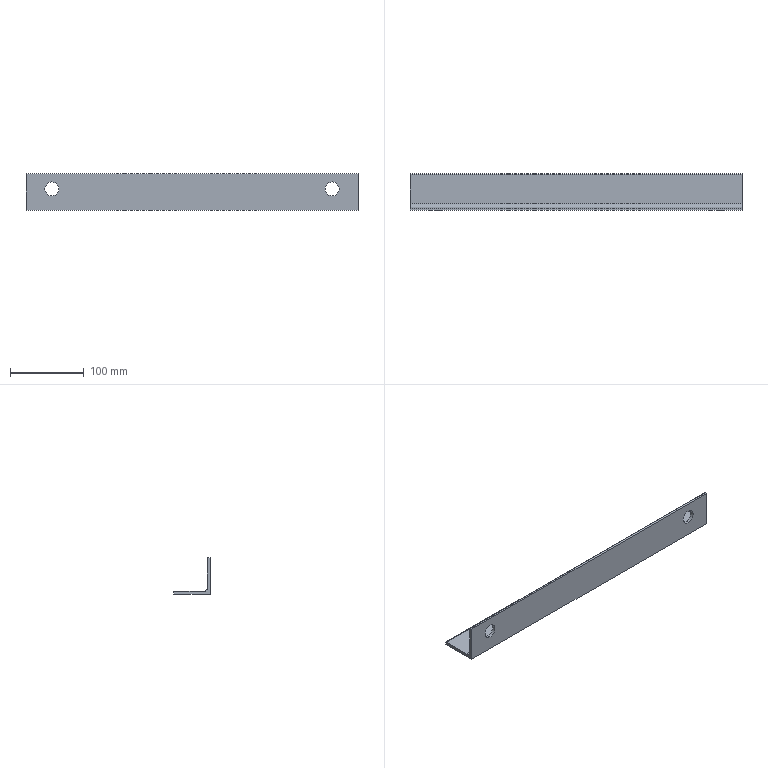Part | STEP file | 计量角钢2_Default<As Machined> | 1 solid | 15 faces | box 450 x 50 x 50 mm | volume 173111 mm3 | plane 8 | cylinder 7 | commonest cylinder face diameters 19 x4 2.66 x2 11 x1
STEP:
#1=CARTESIAN_POINT('',(0.,0.,0.));
#2=DIRECTION('',(0.,0.,1.));
#3=DIRECTION('',(1.,0.,0.));
#4=AXIS2_PLACEMENT_3D('',#1,#2,#3);
#5=CARTESIAN_POINT('',(-190.,0.,38.585));
#6=VERTEX_POINT('',#5);
#7=CARTESIAN_POINT('',(-190.,4.,38.585));
#8=VERTEX_POINT('',#7);
#9=CARTESIAN_POINT('',(-190.,-6.,38.585));
#10=DIRECTION('',(0.,1.,0.));
#11=VECTOR('',#10,1.);
#12=LINE('',#9,#11);
#13=CARTESIAN_POINT('',(-190.,-6.,29.085));
#14=DIRECTION('',(0.,1.,0.));
#15=DIRECTION('',(0.,0.,1.));
#16=AXIS2_PLACEMENT_3D('',#13,#14,#15);
#17=CYLINDRICAL_SURFACE('',#16,9.5);
#18=CARTESIAN_POINT('',(6.283,0.));
#19=DIRECTION('',(0.,1.));
#20=VECTOR('',#19,1.);
#21=LINE('',#18,#20);
#22=(GEOMETRIC_REPRESENTATION_CONTEXT(2)PARAMETRIC_REPRESENTATION_CONTEXT()REPRESENTATION_CONTEXT('',''));
#23=DEFINITIONAL_REPRESENTATION('',(#21),#22);
#24=PCURVE('',#17,#23);
#25=CARTESIAN_POINT('',(-190.,-6.,29.085));
#26=DIRECTION('',(0.,1.,0.));
#27=DIRECTION('',(0.,0.,1.));
#28=AXIS2_PLACEMENT_3D('',#25,#26,#27);
#29=CYLINDRICAL_SURFACE('',#28,9.5);
#30=CARTESIAN_POINT('',(0.,0.));
#31=DIRECTION('',(0.,1.));
#32=VECTOR('',#31,1.);
#33=LINE('',#30,#32);
#34=(GEOMETRIC_REPRESENTATION_CONTEXT(2)PARAMETRIC_REPRESENTATION_CONTEXT()REPRESENTATION_CONTEXT('',''));
#35=DEFINITIONAL_REPRESENTATION('',(#33),#34);
#36=PCURVE('',#29,#35);
#37=SURFACE_CURVE('',#12,(#24,#36),.PCURVE_S1.);
#38=EDGE_CURVE('',#6,#8,#37,.T.);
#39=ORIENTED_EDGE('',*,*,#38,.T.);
#40=CARTESIAN_POINT('',(-190.,4.,19.585));
#41=VERTEX_POINT('',#40);
#42=CARTESIAN_POINT('',(-190.,4.,29.085));
#43=DIRECTION('',(0.,1.,0.));
#44=DIRECTION('',(0.,0.,1.));
#45=AXIS2_PLACEMENT_3D('',#42,#43,#44);
#46=CIRCLE('',#45,9.5);
#47=CARTESIAN_POINT('',(0.,10.));
#48=DIRECTION('',(1.,0.));
#49=VECTOR('',#48,1.);
#50=LINE('',#47,#49);
#51=(GEOMETRIC_REPRESENTATION_CONTEXT(2)PARAMETRIC_REPRESENTATION_CONTEXT()REPRESENTATION_CONTEXT('',''));
#52=DEFINITIONAL_REPRESENTATION('',(#50),#51);
#53=PCURVE('',#17,#52);
#54=CARTESIAN_POINT('',(225.,4.,48.67));
#55=DIRECTION('',(0.,-1.,0.));
#56=DIRECTION('',(1.,0.,0.));
#57=AXIS2_PLACEMENT_3D('',#54,#55,#56);
#58=PLANE('',#57);
#59=CARTESIAN_POINT('',(-415.,-10.085));
#60=CARTESIAN_POINT('',(-398.546,-10.085));
#61=CARTESIAN_POINT('',(-406.773,-24.335));
#62=CARTESIAN_POINT('',(-415.,-38.585));
#63=CARTESIAN_POINT('',(-423.227,-24.335));
#64=CARTESIAN_POINT('',(-431.454,-10.085));
#65=CARTESIAN_POINT('',(-415.,-10.085));
#66=(BOUNDED_CURVE()B_SPLINE_CURVE(2,(#59,#60,#61,#62,#63,#64,#65),.UNSPECIFIED.,.T.,.F.)B_SPLINE_CURVE_WITH_KNOTS((1,2,2,2,2,1),(-2.094,0.,2.094,4.189,6.283,8.378),.UNSPECIFIED.)CURVE()GEOMETRIC_REPRESENTATION_ITEM()RATIONAL_B_SPLINE_CURVE((1.,0.5,1.,0.5,1.,0.5,1.))REPRESENTATION_ITEM(''));
#67=(GEOMETRIC_REPRESENTATION_CONTEXT(2)PARAMETRIC_REPRESENTATION_CONTEXT()REPRESENTATION_CONTEXT('',''));
#68=DEFINITIONAL_REPRESENTATION('',(#66),#67);
#69=PCURVE('',#58,#68);
#70=SURFACE_CURVE('',#46,(#53,#69),.PCURVE_S1.);
#71=EDGE_CURVE('',#41,#8,#70,.T.);
#72=ORIENTED_EDGE('',*,*,#71,.F.);
#73=CARTESIAN_POINT('',(-190.,0.,19.585));
#74=VERTEX_POINT('',#73);
#75=CARTESIAN_POINT('',(-190.,-6.,19.585));
#76=DIRECTION('',(0.,1.,0.));
#77=VECTOR('',#76,1.);
#78=LINE('',#75,#77);
#79=CARTESIAN_POINT('',(3.142,0.));
#80=DIRECTION('',(0.,1.));
#81=VECTOR('',#80,1.);
#82=LINE('',#79,#81);
#83=(GEOMETRIC_REPRESENTATION_CONTEXT(2)PARAMETRIC_REPRESENTATION_CONTEXT()REPRESENTATION_CONTEXT('',''));
#84=DEFINITIONAL_REPRESENTATION('',(#82),#83);
#85=PCURVE('',#17,#84);
#86=CARTESIAN_POINT('',(3.142,0.));
#87=DIRECTION('',(0.,1.));
#88=VECTOR('',#87,1.);
#89=LINE('',#86,#88);
#90=(GEOMETRIC_REPRESENTATION_CONTEXT(2)PARAMETRIC_REPRESENTATION_CONTEXT()REPRESENTATION_CONTEXT('',''));
#91=DEFINITIONAL_REPRESENTATION('',(#89),#90);
#92=PCURVE('',#29,#91);
#93=SURFACE_CURVE('',#78,(#85,#92),.PCURVE_S1.);
#94=EDGE_CURVE('',#74,#41,#93,.T.);
#95=ORIENTED_EDGE('',*,*,#94,.F.);
#96=CARTESIAN_POINT('',(-190.,0.,29.085));
#97=DIRECTION('',(0.,1.,0.));
#98=DIRECTION('',(-1.,0.,0.));
#99=AXIS2_PLACEMENT_3D('',#96,#97,#98);
#100=CIRCLE('',#99,9.5);
#101=CARTESIAN_POINT('',(-1.571,6.));
#102=DIRECTION('',(1.,0.));
#103=VECTOR('',#102,1.);
#104=LINE('',#101,#103);
#105=(GEOMETRIC_REPRESENTATION_CONTEXT(2)PARAMETRIC_REPRESENTATION_CONTEXT()REPRESENTATION_CONTEXT('',''));
#106=DEFINITIONAL_REPRESENTATION('',(#104),#105);
#107=PCURVE('',#17,#106);
#108=CARTESIAN_POINT('',(225.,0.,50.));
#109=DIRECTION('',(0.,1.,0.));
#110=DIRECTION('',(-1.,0.,0.));
#111=AXIS2_PLACEMENT_3D('',#108,#109,#110);
#112=PLANE('',#111);
#113=CARTESIAN_POINT('',(415.,-20.915));
#114=DIRECTION('',(1.,0.));
#115=AXIS2_PLACEMENT_2D('',#113,#114);
#116=CIRCLE('',#115,9.5);
#117=(GEOMETRIC_REPRESENTATION_CONTEXT(2)PARAMETRIC_REPRESENTATION_CONTEXT()REPRESENTATION_CONTEXT('',''));
#118=DEFINITIONAL_REPRESENTATION('',(#116),#117);
#119=PCURVE('',#112,#118);
#120=SURFACE_CURVE('',#100,(#107,#119),.PCURVE_S1.);
#121=EDGE_CURVE('',#74,#6,#120,.T.);
#122=ORIENTED_EDGE('',*,*,#121,.T.);
#123=EDGE_LOOP('',(#39,#72,#95,#122));
#124=FACE_BOUND('',#123,.F.);
#125=ADVANCED_FACE('',(#124),#17,.F.);
#126=CARTESIAN_POINT('',(190.,0.,38.585));
#127=VERTEX_POINT('',#126);
#128=CARTESIAN_POINT('',(190.,4.,38.585));
#129=VERTEX_POINT('',#128);
#130=CARTESIAN_POINT('',(190.,-6.,38.585));
#131=DIRECTION('',(0.,1.,0.));
#132=VECTOR('',#131,1.);
#133=LINE('',#130,#132);
#134=CARTESIAN_POINT('',(190.,-6.,29.085));
#135=DIRECTION('',(0.,1.,0.));
#136=DIRECTION('',(0.,0.,1.));
#137=AXIS2_PLACEMENT_3D('',#134,#135,#136);
#138=CYLINDRICAL_SURFACE('',#137,9.5);
#139=CARTESIAN_POINT('',(6.283,0.));
#140=DIRECTION('',(0.,1.));
#141=VECTOR('',#140,1.);
#142=LINE('',#139,#141);
#143=(GEOMETRIC_REPRESENTATION_CONTEXT(2)PARAMETRIC_REPRESENTATION_CONTEXT()REPRESENTATION_CONTEXT('',''));
#144=DEFINITIONAL_REPRESENTATION('',(#142),#143);
#145=PCURVE('',#138,#144);
#146=CARTESIAN_POINT('',(190.,-6.,29.085));
#147=DIRECTION('',(0.,1.,0.));
#148=DIRECTION('',(0.,0.,1.));
#149=AXIS2_PLACEMENT_3D('',#146,#147,#148);
#150=CYLINDRICAL_SURFACE('',#149,9.5);
#151=CARTESIAN_POINT('',(0.,0.));
#152=DIRECTION('',(0.,1.));
#153=VECTOR('',#152,1.);
#154=LINE('',#151,#153);
#155=(GEOMETRIC_REPRESENTATION_CONTEXT(2)PARAMETRIC_REPRESENTATION_CONTEXT()REPRESENTATION_CONTEXT('',''));
#156=DEFINITIONAL_REPRESENTATION('',(#154),#155);
#157=PCURVE('',#150,#156);
#158=SURFACE_CURVE('',#133,(#145,#157),.PCURVE_S1.);
#159=EDGE_CURVE('',#127,#129,#158,.T.);
#160=ORIENTED_EDGE('',*,*,#159,.T.);
#161=CARTESIAN_POINT('',(190.,4.,19.585));
#162=VERTEX_POINT('',#161);
#163=CARTESIAN_POINT('',(190.,4.,29.085));
#164=DIRECTION('',(0.,1.,0.));
#165=DIRECTION('',(0.,0.,-1.));
#166=AXIS2_PLACEMENT_3D('',#163,#164,#165);
#167=CIRCLE('',#166,9.5);
#168=CARTESIAN_POINT('',(3.142,10.));
#169=DIRECTION('',(1.,0.));
#170=VECTOR('',#169,1.);
#171=LINE('',#168,#170);
#172=(GEOMETRIC_REPRESENTATION_CONTEXT(2)PARAMETRIC_REPRESENTATION_CONTEXT()REPRESENTATION_CONTEXT('',''));
#173=DEFINITIONAL_REPRESENTATION('',(#171),#172);
#174=PCURVE('',#138,#173);
#175=CARTESIAN_POINT('',(-35.,-29.085));
#176=CARTESIAN_POINT('',(-51.454,-29.085));
#177=CARTESIAN_POINT('',(-43.227,-14.835));
#178=CARTESIAN_POINT('',(-35.,-0.585));
#179=CARTESIAN_POINT('',(-26.773,-14.835));
#180=CARTESIAN_POINT('',(-18.546,-29.085));
#181=CARTESIAN_POINT('',(-35.,-29.085));
#182=(BOUNDED_CURVE()B_SPLINE_CURVE(2,(#175,#176,#177,#178,#179,#180,#181),.UNSPECIFIED.,.T.,.F.)B_SPLINE_CURVE_WITH_KNOTS((1,2,2,2,2,1),(-2.094,0.,2.094,4.189,6.283,8.378),.UNSPECIFIED.)CURVE()GEOMETRIC_REPRESENTATION_ITEM()RATIONAL_B_SPLINE_CURVE((1.,0.5,1.,0.5,1.,0.5,1.))REPRESENTATION_ITEM(''));
#183=(GEOMETRIC_REPRESENTATION_CONTEXT(2)PARAMETRIC_REPRESENTATION_CONTEXT()REPRESENTATION_CONTEXT('',''));
#184=DEFINITIONAL_REPRESENTATION('',(#182),#183);
#185=PCURVE('',#58,#184);
#186=SURFACE_CURVE('',#167,(#174,#185),.PCURVE_S1.);
#187=EDGE_CURVE('',#162,#129,#186,.T.);
#188=ORIENTED_EDGE('',*,*,#187,.F.);
#189=CARTESIAN_POINT('',(190.,0.,19.585));
#190=VERTEX_POINT('',#189);
#191=CARTESIAN_POINT('',(190.,-6.,19.585));
#192=DIRECTION('',(0.,1.,0.));
#193=VECTOR('',#192,1.);
#194=LINE('',#191,#193);
#195=CARTESIAN_POINT('',(3.142,0.));
#196=DIRECTION('',(0.,1.));
#197=VECTOR('',#196,1.);
#198=LINE('',#195,#197);
#199=(GEOMETRIC_REPRESENTATION_CONTEXT(2)PARAMETRIC_REPRESENTATION_CONTEXT()REPRESENTATION_CONTEXT('',''));
#200=DEFINITIONAL_REPRESENTATION('',(#198),#199);
#201=PCURVE('',#138,#200);
#202=CARTESIAN_POINT('',(3.142,0.));
#203=DIRECTION('',(0.,1.));
#204=VECTOR('',#203,1.);
#205=LINE('',#202,#204);
#206=(GEOMETRIC_REPRESENTATION_CONTEXT(2)PARAMETRIC_REPRESENTATION_CONTEXT()REPRESENTATION_CONTEXT('',''));
#207=DEFINITIONAL_REPRESENTATION('',(#205),#206);
#208=PCURVE('',#150,#207);
#209=SURFACE_CURVE('',#194,(#201,#208),.PCURVE_S1.);
#210=EDGE_CURVE('',#190,#162,#209,.T.);
#211=ORIENTED_EDGE('',*,*,#210,.F.);
#212=CARTESIAN_POINT('',(190.,0.,29.085));
#213=DIRECTION('',(0.,1.,0.));
#214=DIRECTION('',(-1.,0.,0.));
#215=AXIS2_PLACEMENT_3D('',#212,#213,#214);
#216=CIRCLE('',#215,9.5);
#217=CARTESIAN_POINT('',(-1.571,6.));
#218=DIRECTION('',(1.,0.));
#219=VECTOR('',#218,1.);
#220=LINE('',#217,#219);
#221=(GEOMETRIC_REPRESENTATION_CONTEXT(2)PARAMETRIC_REPRESENTATION_CONTEXT()REPRESENTATION_CONTEXT('',''));
#222=DEFINITIONAL_REPRESENTATION('',(#220),#221);
#223=PCURVE('',#138,#222);
#224=CARTESIAN_POINT('',(35.,-20.915));
#225=DIRECTION('',(1.,0.));
#226=AXIS2_PLACEMENT_2D('',#224,#225);
#227=CIRCLE('',#226,9.5);
#228=(GEOMETRIC_REPRESENTATION_CONTEXT(2)PARAMETRIC_REPRESENTATION_CONTEXT()REPRESENTATION_CONTEXT('',''));
#229=DEFINITIONAL_REPRESENTATION('',(#227),#228);
#230=PCURVE('',#112,#229);
#231=SURFACE_CURVE('',#216,(#223,#230),.PCURVE_S1.);
#232=EDGE_CURVE('',#190,#127,#231,.T.);
#233=ORIENTED_EDGE('',*,*,#232,.T.);
#234=EDGE_LOOP('',(#160,#188,#211,#233));
#235=FACE_BOUND('',#234,.F.);
#236=ADVANCED_FACE('',(#235),#138,.F.);
#237=CARTESIAN_POINT('',(-225.,50.,2.67));
#238=VERTEX_POINT('',#237);
#239=CARTESIAN_POINT('',(-225.,48.67,4.));
#240=VERTEX_POINT('',#239);
#241=CARTESIAN_POINT('',(-225.,48.67,2.67));
#242=DIRECTION('',(1.,0.,0.));
#243=DIRECTION('',(0.,1.,0.));
#244=AXIS2_PLACEMENT_3D('',#241,#242,#243);
#245=CIRCLE('',#244,1.33);
#246=CARTESIAN_POINT('',(225.,48.67,2.67));
#247=DIRECTION('',(-1.,0.,0.));
#248=DIRECTION('',(0.,-1.,0.));
#249=AXIS2_PLACEMENT_3D('',#246,#247,#248);
#250=CYLINDRICAL_SURFACE('',#249,1.33);
#251=CARTESIAN_POINT('',(3.142,450.));
#252=DIRECTION('',(-1.,0.));
#253=VECTOR('',#252,1.);
#254=LINE('',#251,#253);
#255=(GEOMETRIC_REPRESENTATION_CONTEXT(2)PARAMETRIC_REPRESENTATION_CONTEXT()REPRESENTATION_CONTEXT('',''));
#256=DEFINITIONAL_REPRESENTATION('',(#254),#255);
#257=PCURVE('',#250,#256);
#258=CARTESIAN_POINT('',(-225.,48.67,2.67));
#259=DIRECTION('',(1.,0.,0.));
#260=DIRECTION('',(0.,1.,0.));
#261=AXIS2_PLACEMENT_3D('',#258,#259,#260);
#262=PLANE('',#261);
#263=CARTESIAN_POINT('',(0.,0.));
#264=DIRECTION('',(1.,0.));
#265=AXIS2_PLACEMENT_2D('',#263,#264);
#266=CIRCLE('',#265,1.33);
#267=(GEOMETRIC_REPRESENTATION_CONTEXT(2)PARAMETRIC_REPRESENTATION_CONTEXT()REPRESENTATION_CONTEXT('',''));
#268=DEFINITIONAL_REPRESENTATION('',(#266),#267);
#269=PCURVE('',#262,#268);
#270=SURFACE_CURVE('',#245,(#257,#269),.PCURVE_S1.);
#271=EDGE_CURVE('',#238,#240,#270,.T.);
#272=ORIENTED_EDGE('',*,*,#271,.T.);
#273=CARTESIAN_POINT('',(225.,48.67,4.));
#274=VERTEX_POINT('',#273);
#275=CARTESIAN_POINT('',(225.,48.67,4.));
#276=DIRECTION('',(-1.,0.,0.));
#277=VECTOR('',#276,1.);
#278=LINE('',#275,#277);
#279=CARTESIAN_POINT('',(1.571,0.));
#280=DIRECTION('',(0.,1.));
#281=VECTOR('',#280,1.);
#282=LINE('',#279,#281);
#283=(GEOMETRIC_REPRESENTATION_CONTEXT(2)PARAMETRIC_REPRESENTATION_CONTEXT()REPRESENTATION_CONTEXT('',''));
#284=DEFINITIONAL_REPRESENTATION('',(#282),#283);
#285=PCURVE('',#250,#284);
#286=CARTESIAN_POINT('',(225.,9.5,4.));
#287=DIRECTION('',(0.,0.,-1.));
#288=DIRECTION('',(-1.,0.,0.));
#289=AXIS2_PLACEMENT_3D('',#286,#287,#288);
#290=PLANE('',#289);
#291=CARTESIAN_POINT('',(0.,39.17));
#292=DIRECTION('',(1.,0.));
#293=VECTOR('',#292,1.);
#294=LINE('',#291,#293);
#295=(GEOMETRIC_REPRESENTATION_CONTEXT(2)PARAMETRIC_REPRESENTATION_CONTEXT()REPRESENTATION_CONTEXT('',''));
#296=DEFINITIONAL_REPRESENTATION('',(#294),#295);
#297=PCURVE('',#290,#296);
#298=SURFACE_CURVE('',#278,(#285,#297),.PCURVE_S1.);
#299=EDGE_CURVE('',#274,#240,#298,.T.);
#300=ORIENTED_EDGE('',*,*,#299,.F.);
#301=CARTESIAN_POINT('',(225.,50.,2.67));
#302=VERTEX_POINT('',#301);
#303=CARTESIAN_POINT('',(225.,48.67,2.67));
#304=DIRECTION('',(1.,0.,0.));
#305=DIRECTION('',(0.,1.,0.));
#306=AXIS2_PLACEMENT_3D('',#303,#304,#305);
#307=CIRCLE('',#306,1.33);
#308=CARTESIAN_POINT('',(3.142,0.));
#309=DIRECTION('',(-1.,0.));
#310=VECTOR('',#309,1.);
#311=LINE('',#308,#310);
#312=(GEOMETRIC_REPRESENTATION_CONTEXT(2)PARAMETRIC_REPRESENTATION_CONTEXT()REPRESENTATION_CONTEXT('',''));
#313=DEFINITIONAL_REPRESENTATION('',(#311),#312);
#314=PCURVE('',#250,#313);
#315=CARTESIAN_POINT('',(225.,48.67,2.67));
#316=DIRECTION('',(1.,0.,0.));
#317=DIRECTION('',(0.,1.,0.));
#318=AXIS2_PLACEMENT_3D('',#315,#316,#317);
#319=PLANE('',#318);
#320=CARTESIAN_POINT('',(0.,0.));
#321=DIRECTION('',(1.,0.));
#322=AXIS2_PLACEMENT_2D('',#320,#321);
#323=CIRCLE('',#322,1.33);
#324=(GEOMETRIC_REPRESENTATION_CONTEXT(2)PARAMETRIC_REPRESENTATION_CONTEXT()REPRESENTATION_CONTEXT('',''));
#325=DEFINITIONAL_REPRESENTATION('',(#323),#324);
#326=PCURVE('',#319,#325);
#327=SURFACE_CURVE('',#307,(#314,#326),.PCURVE_S1.);
#328=EDGE_CURVE('',#302,#274,#327,.T.);
#329=ORIENTED_EDGE('',*,*,#328,.F.);
#330=CARTESIAN_POINT('',(225.,50.,2.67));
#331=DIRECTION('',(-1.,0.,0.));
#332=VECTOR('',#331,1.);
#333=LINE('',#330,#332);
#334=CARTESIAN_POINT('',(3.142,0.));
#335=DIRECTION('',(0.,1.));
#336=VECTOR('',#335,1.);
#337=LINE('',#334,#336);
#338=(GEOMETRIC_REPRESENTATION_CONTEXT(2)PARAMETRIC_REPRESENTATION_CONTEXT()REPRESENTATION_CONTEXT('',''));
#339=DEFINITIONAL_REPRESENTATION('',(#337),#338);
#340=PCURVE('',#250,#339);
#341=CARTESIAN_POINT('',(225.,50.,2.67));
#342=DIRECTION('',(0.,-1.,0.));
#343=DIRECTION('',(1.,0.,0.));
#344=AXIS2_PLACEMENT_3D('',#341,#342,#343);
#345=PLANE('',#344);
#346=CARTESIAN_POINT('',(0.,0.));
#347=DIRECTION('',(-1.,0.));
#348=VECTOR('',#347,1.);
#349=LINE('',#346,#348);
#350=(GEOMETRIC_REPRESENTATION_CONTEXT(2)PARAMETRIC_REPRESENTATION_CONTEXT()REPRESENTATION_CONTEXT('',''));
#351=DEFINITIONAL_REPRESENTATION('',(#349),#350);
#352=PCURVE('',#345,#351);
#353=SURFACE_CURVE('',#333,(#340,#352),.PCURVE_S1.);
#354=EDGE_CURVE('',#302,#238,#353,.T.);
#355=ORIENTED_EDGE('',*,*,#354,.T.);
#356=EDGE_LOOP('',(#272,#300,#329,#355));
#357=FACE_BOUND('',#356,.T.);
#358=ADVANCED_FACE('',(#357),#250,.T.);
#359=CARTESIAN_POINT('',(-225.,9.5,4.));
#360=VERTEX_POINT('',#359);
#361=CARTESIAN_POINT('',(-225.,9.5,4.));
#362=DIRECTION('',(0.,-1.,0.));
#363=VECTOR('',#362,1.);
#364=LINE('',#361,#363);
#365=CARTESIAN_POINT('',(450.,0.));
#366=DIRECTION('',(0.,-1.));
#367=VECTOR('',#366,1.);
#368=LINE('',#365,#367);
#369=(GEOMETRIC_REPRESENTATION_CONTEXT(2)PARAMETRIC_REPRESENTATION_CONTEXT()REPRESENTATION_CONTEXT('',''));
#370=DEFINITIONAL_REPRESENTATION('',(#368),#369);
#371=PCURVE('',#290,#370);
#372=CARTESIAN_POINT('',(-39.17,1.33));
#373=DIRECTION('',(-1.,0.));
#374=VECTOR('',#373,1.);
#375=LINE('',#372,#374);
#376=(GEOMETRIC_REPRESENTATION_CONTEXT(2)PARAMETRIC_REPRESENTATION_CONTEXT()REPRESENTATION_CONTEXT('',''));
#377=DEFINITIONAL_REPRESENTATION('',(#375),#376);
#378=PCURVE('',#262,#377);
#379=SURFACE_CURVE('',#364,(#371,#378),.PCURVE_S1.);
#380=EDGE_CURVE('',#240,#360,#379,.T.);
#381=ORIENTED_EDGE('',*,*,#380,.T.);
#382=CARTESIAN_POINT('',(225.,9.5,4.));
#383=VERTEX_POINT('',#382);
#384=CARTESIAN_POINT('',(225.,9.5,4.));
#385=DIRECTION('',(-1.,0.,0.));
#386=VECTOR('',#385,1.);
#387=LINE('',#384,#386);
#388=CARTESIAN_POINT('',(0.,0.));
#389=DIRECTION('',(1.,0.));
#390=VECTOR('',#389,1.);
#391=LINE('',#388,#390);
#392=(GEOMETRIC_REPRESENTATION_CONTEXT(2)PARAMETRIC_REPRESENTATION_CONTEXT()REPRESENTATION_CONTEXT('',''));
#393=DEFINITIONAL_REPRESENTATION('',(#391),#392);
#394=PCURVE('',#290,#393);
#395=CARTESIAN_POINT('',(225.,9.5,9.5));
#396=DIRECTION('',(-1.,0.,0.));
#397=DIRECTION('',(0.,-1.,0.));
#398=AXIS2_PLACEMENT_3D('',#395,#396,#397);
#399=CYLINDRICAL_SURFACE('',#398,5.5);
#400=CARTESIAN_POINT('',(4.712,0.));
#401=DIRECTION('',(0.,1.));
#402=VECTOR('',#401,1.);
#403=LINE('',#400,#402);
#404=(GEOMETRIC_REPRESENTATION_CONTEXT(2)PARAMETRIC_REPRESENTATION_CONTEXT()REPRESENTATION_CONTEXT('',''));
#405=DEFINITIONAL_REPRESENTATION('',(#403),#404);
#406=PCURVE('',#399,#405);
#407=SURFACE_CURVE('',#387,(#394,#406),.PCURVE_S1.);
#408=EDGE_CURVE('',#383,#360,#407,.T.);
#409=ORIENTED_EDGE('',*,*,#408,.F.);
#410=CARTESIAN_POINT('',(225.,9.5,4.));
#411=DIRECTION('',(0.,-1.,0.));
#412=VECTOR('',#411,1.);
#413=LINE('',#410,#412);
#414=CARTESIAN_POINT('',(0.,0.));
#415=DIRECTION('',(0.,-1.));
#416=VECTOR('',#415,1.);
#417=LINE('',#414,#416);
#418=(GEOMETRIC_REPRESENTATION_CONTEXT(2)PARAMETRIC_REPRESENTATION_CONTEXT()REPRESENTATION_CONTEXT('',''));
#419=DEFINITIONAL_REPRESENTATION('',(#417),#418);
#420=PCURVE('',#290,#419);
#421=CARTESIAN_POINT('',(-39.17,1.33));
#422=DIRECTION('',(-1.,0.));
#423=VECTOR('',#422,1.);
#424=LINE('',#421,#423);
#425=(GEOMETRIC_REPRESENTATION_CONTEXT(2)PARAMETRIC_REPRESENTATION_CONTEXT()REPRESENTATION_CONTEXT('',''));
#426=DEFINITIONAL_REPRESENTATION('',(#424),#425);
#427=PCURVE('',#319,#426);
#428=SURFACE_CURVE('',#413,(#420,#427),.PCURVE_S1.);
#429=EDGE_CURVE('',#274,#383,#428,.T.);
#430=ORIENTED_EDGE('',*,*,#429,.F.);
#431=ORIENTED_EDGE('',*,*,#299,.T.);
#432=EDGE_LOOP('',(#381,#409,#430,#431));
#433=FACE_BOUND('',#432,.T.);
#434=ADVANCED_FACE('',(#433),#290,.F.);
#435=ORIENTED_EDGE('',*,*,#408,.F.);
#436=CARTESIAN_POINT('',(225.,4.,9.5));
#437=VERTEX_POINT('',#436);
#438=CARTESIAN_POINT('',(225.,9.5,9.5));
#439=DIRECTION('',(-1.,0.,0.));
#440=DIRECTION('',(0.,1.,0.));
#441=AXIS2_PLACEMENT_3D('',#438,#439,#440);
#442=CIRCLE('',#441,5.5);
#443=CARTESIAN_POINT('',(3.142,0.));
#444=DIRECTION('',(1.,0.));
#445=VECTOR('',#444,1.);
#446=LINE('',#443,#445);
#447=(GEOMETRIC_REPRESENTATION_CONTEXT(2)PARAMETRIC_REPRESENTATION_CONTEXT()REPRESENTATION_CONTEXT('',''));
#448=DEFINITIONAL_REPRESENTATION('',(#446),#447);
#449=PCURVE('',#399,#448);
#450=CARTESIAN_POINT('',(-33.67,6.83));
#451=CARTESIAN_POINT('',(-33.67,-2.696));
#452=CARTESIAN_POINT('',(-41.92,2.067));
#453=CARTESIAN_POINT('',(-50.17,6.83));
#454=CARTESIAN_POINT('',(-41.92,11.593));
#455=CARTESIAN_POINT('',(-33.67,16.356));
#456=CARTESIAN_POINT('',(-33.67,6.83));
#457=(BOUNDED_CURVE()B_SPLINE_CURVE(2,(#450,#451,#452,#453,#454,#455,#456),.UNSPECIFIED.,.T.,.F.)B_SPLINE_CURVE_WITH_KNOTS((1,2,2,2,2,1),(-2.094,0.,2.094,4.189,6.283,8.378),.UNSPECIFIED.)CURVE()GEOMETRIC_REPRESENTATION_ITEM()RATIONAL_B_SPLINE_CURVE((1.,0.5,1.,0.5,1.,0.5,1.))REPRESENTATION_ITEM(''));
#458=(GEOMETRIC_REPRESENTATION_CONTEXT(2)PARAMETRIC_REPRESENTATION_CONTEXT()REPRESENTATION_CONTEXT('',''));
#459=DEFINITIONAL_REPRESENTATION('',(#457),#458);
#460=PCURVE('',#319,#459);
#461=SURFACE_CURVE('',#442,(#449,#460),.PCURVE_S1.);
#462=EDGE_CURVE('',#383,#437,#461,.T.);
#463=ORIENTED_EDGE('',*,*,#462,.T.);
#464=CARTESIAN_POINT('',(-225.,4.,9.5));
#465=VERTEX_POINT('',#464);
#466=CARTESIAN_POINT('',(225.,4.,9.5));
#467=DIRECTION('',(-1.,0.,0.));
#468=VECTOR('',#467,1.);
#469=LINE('',#466,#468);
#470=CARTESIAN_POINT('',(6.283,0.));
#471=DIRECTION('',(0.,1.));
#472=VECTOR('',#471,1.);
#473=LINE('',#470,#472);
#474=(GEOMETRIC_REPRESENTATION_CONTEXT(2)PARAMETRIC_REPRESENTATION_CONTEXT()REPRESENTATION_CONTEXT('',''));
#475=DEFINITIONAL_REPRESENTATION('',(#473),#474);
#476=PCURVE('',#399,#475);
#477=CARTESIAN_POINT('',(0.,-39.17));
#478=DIRECTION('',(-1.,0.));
#479=VECTOR('',#478,1.);
#480=LINE('',#477,#479);
#481=(GEOMETRIC_REPRESENTATION_CONTEXT(2)PARAMETRIC_REPRESENTATION_CONTEXT()REPRESENTATION_CONTEXT('',''));
#482=DEFINITIONAL_REPRESENTATION('',(#480),#481);
#483=PCURVE('',#58,#482);
#484=SURFACE_CURVE('',#469,(#476,#483),.PCURVE_S1.);
#485=EDGE_CURVE('',#437,#465,#484,.T.);
#486=ORIENTED_EDGE('',*,*,#485,.T.);
#487=CARTESIAN_POINT('',(-225.,9.5,9.5));
#488=DIRECTION('',(-1.,0.,0.));
#489=DIRECTION('',(0.,1.,0.));
#490=AXIS2_PLACEMENT_3D('',#487,#488,#489);
#491=CIRCLE('',#490,5.5);
#492=CARTESIAN_POINT('',(3.142,450.));
#493=DIRECTION('',(1.,0.));
#494=VECTOR('',#493,1.);
#495=LINE('',#492,#494);
#496=(GEOMETRIC_REPRESENTATION_CONTEXT(2)PARAMETRIC_REPRESENTATION_CONTEXT()REPRESENTATION_CONTEXT('',''));
#497=DEFINITIONAL_REPRESENTATION('',(#495),#496);
#498=PCURVE('',#399,#497);
#499=CARTESIAN_POINT('',(-33.67,6.83));
#500=CARTESIAN_POINT('',(-33.67,-2.696));
#501=CARTESIAN_POINT('',(-41.92,2.067));
#502=CARTESIAN_POINT('',(-50.17,6.83));
#503=CARTESIAN_POINT('',(-41.92,11.593));
#504=CARTESIAN_POINT('',(-33.67,16.356));
#505=CARTESIAN_POINT('',(-33.67,6.83));
#506=(BOUNDED_CURVE()B_SPLINE_CURVE(2,(#499,#500,#501,#502,#503,#504,#505),.UNSPECIFIED.,.T.,.F.)B_SPLINE_CURVE_WITH_KNOTS((1,2,2,2,2,1),(-2.094,0.,2.094,4.189,6.283,8.378),.UNSPECIFIED.)CURVE()GEOMETRIC_REPRESENTATION_ITEM()RATIONAL_B_SPLINE_CURVE((1.,0.5,1.,0.5,1.,0.5,1.))REPRESENTATION_ITEM(''));
#507=(GEOMETRIC_REPRESENTATION_CONTEXT(2)PARAMETRIC_REPRESENTATION_CONTEXT()REPRESENTATION_CONTEXT('',''));
#508=DEFINITIONAL_REPRESENTATION('',(#506),#507);
#509=PCURVE('',#262,#508);
#510=SURFACE_CURVE('',#491,(#498,#509),.PCURVE_S1.);
#511=EDGE_CURVE('',#360,#465,#510,.T.);
#512=ORIENTED_EDGE('',*,*,#511,.F.);
#513=EDGE_LOOP('',(#435,#463,#486,#512));
#514=FACE_BOUND('',#513,.F.);
#515=ADVANCED_FACE('',(#514),#399,.F.);
#516=CARTESIAN_POINT('',(-190.,4.,29.085));
#517=DIRECTION('',(0.,1.,0.));
#518=DIRECTION('',(0.,0.,1.));
#519=AXIS2_PLACEMENT_3D('',#516,#517,#518);
#520=CIRCLE('',#519,9.5);
#521=CARTESIAN_POINT('',(-415.,-10.085));
#522=CARTESIAN_POINT('',(-398.546,-10.085));
#523=CARTESIAN_POINT('',(-406.773,-24.335));
#524=CARTESIAN_POINT('',(-415.,-38.585));
#525=CARTESIAN_POINT('',(-423.227,-24.335));
#526=CARTESIAN_POINT('',(-431.454,-10.085));
#527=CARTESIAN_POINT('',(-415.,-10.085));
#528=(BOUNDED_CURVE()B_SPLINE_CURVE(2,(#521,#522,#523,#524,#525,#526,#527),.UNSPECIFIED.,.T.,.F.)B_SPLINE_CURVE_WITH_KNOTS((1,2,2,2,2,1),(-2.094,0.,2.094,4.189,6.283,8.378),.UNSPECIFIED.)CURVE()GEOMETRIC_REPRESENTATION_ITEM()RATIONAL_B_SPLINE_CURVE((1.,0.5,1.,0.5,1.,0.5,1.))REPRESENTATION_ITEM(''));
#529=(GEOMETRIC_REPRESENTATION_CONTEXT(2)PARAMETRIC_REPRESENTATION_CONTEXT()REPRESENTATION_CONTEXT('',''));
#530=DEFINITIONAL_REPRESENTATION('',(#528),#529);
#531=PCURVE('',#58,#530);
#532=CARTESIAN_POINT('',(0.,10.));
#533=DIRECTION('',(1.,0.));
#534=VECTOR('',#533,1.);
#535=LINE('',#532,#534);
#536=(GEOMETRIC_REPRESENTATION_CONTEXT(2)PARAMETRIC_REPRESENTATION_CONTEXT()REPRESENTATION_CONTEXT('',''));
#537=DEFINITIONAL_REPRESENTATION('',(#535),#536);
#538=PCURVE('',#29,#537);
#539=SURFACE_CURVE('',#520,(#531,#538),.PCURVE_S1.);
#540=EDGE_CURVE('',#8,#41,#539,.T.);
#541=ORIENTED_EDGE('',*,*,#540,.F.);
#542=ORIENTED_EDGE('',*,*,#71,.F.);
#543=EDGE_LOOP('',(#541,#542));
#544=FACE_BOUND('',#543,.T.);
#545=CARTESIAN_POINT('',(190.,4.,29.085));
#546=DIRECTION('',(0.,1.,0.));
#547=DIRECTION('',(0.,0.,-1.));
#548=AXIS2_PLACEMENT_3D('',#545,#546,#547);
#549=CIRCLE('',#548,9.5);
#550=CARTESIAN_POINT('',(-35.,-29.085));
#551=CARTESIAN_POINT('',(-51.454,-29.085));
#552=CARTESIAN_POINT('',(-43.227,-14.835));
#553=CARTESIAN_POINT('',(-35.,-0.585));
#554=CARTESIAN_POINT('',(-26.773,-14.835));
#555=CARTESIAN_POINT('',(-18.546,-29.085));
#556=CARTESIAN_POINT('',(-35.,-29.085));
#557=(BOUNDED_CURVE()B_SPLINE_CURVE(2,(#550,#551,#552,#553,#554,#555,#556),.UNSPECIFIED.,.T.,.F.)B_SPLINE_CURVE_WITH_KNOTS((1,2,2,2,2,1),(-2.094,0.,2.094,4.189,6.283,8.378),.UNSPECIFIED.)CURVE()GEOMETRIC_REPRESENTATION_ITEM()RATIONAL_B_SPLINE_CURVE((1.,0.5,1.,0.5,1.,0.5,1.))REPRESENTATION_ITEM(''));
#558=(GEOMETRIC_REPRESENTATION_CONTEXT(2)PARAMETRIC_REPRESENTATION_CONTEXT()REPRESENTATION_CONTEXT('',''));
#559=DEFINITIONAL_REPRESENTATION('',(#557),#558);
#560=PCURVE('',#58,#559);
#561=CARTESIAN_POINT('',(-3.142,10.));
#562=DIRECTION('',(1.,0.));
#563=VECTOR('',#562,1.);
#564=LINE('',#561,#563);
#565=(GEOMETRIC_REPRESENTATION_CONTEXT(2)PARAMETRIC_REPRESENTATION_CONTEXT()REPRESENTATION_CONTEXT('',''));
#566=DEFINITIONAL_REPRESENTATION('',(#564),#565);
#567=PCURVE('',#150,#566);
#568=SURFACE_CURVE('',#549,(#560,#567),.PCURVE_S1.);
#569=EDGE_CURVE('',#129,#162,#568,.T.);
#570=ORIENTED_EDGE('',*,*,#569,.F.);
#571=ORIENTED_EDGE('',*,*,#187,.F.);
#572=EDGE_LOOP('',(#570,#571));
#573=FACE_BOUND('',#572,.T.);
#574=CARTESIAN_POINT('',(-225.,4.,48.67));
#575=VERTEX_POINT('',#574);
#576=CARTESIAN_POINT('',(-225.,4.,48.67));
#577=DIRECTION('',(0.,0.,1.));
#578=VECTOR('',#577,1.);
#579=LINE('',#576,#578);
#580=CARTESIAN_POINT('',(-450.,0.));
#581=DIRECTION('',(0.,1.));
#582=VECTOR('',#581,1.);
#583=LINE('',#580,#582);
#584=(GEOMETRIC_REPRESENTATION_CONTEXT(2)PARAMETRIC_REPRESENTATION_CONTEXT()REPRESENTATION_CONTEXT('',''));
#585=DEFINITIONAL_REPRESENTATION('',(#583),#584);
#586=PCURVE('',#58,#585);
#587=CARTESIAN_POINT('',(-44.67,46.));
#588=DIRECTION('',(0.,1.));
#589=VECTOR('',#588,1.);
#590=LINE('',#587,#589);
#591=(GEOMETRIC_REPRESENTATION_CONTEXT(2)PARAMETRIC_REPRESENTATION_CONTEXT()REPRESENTATION_CONTEXT('',''));
#592=DEFINITIONAL_REPRESENTATION('',(#590),#591);
#593=PCURVE('',#262,#592);
#594=SURFACE_CURVE('',#579,(#586,#593),.PCURVE_S1.);
#595=EDGE_CURVE('',#465,#575,#594,.T.);
#596=ORIENTED_EDGE('',*,*,#595,.T.);
#597=CARTESIAN_POINT('',(225.,4.,48.67));
#598=VERTEX_POINT('',#597);
#599=CARTESIAN_POINT('',(225.,4.,48.67));
#600=DIRECTION('',(-1.,0.,0.));
#601=VECTOR('',#600,1.);
#602=LINE('',#599,#601);
#603=CARTESIAN_POINT('',(0.,0.));
#604=DIRECTION('',(-1.,0.));
#605=VECTOR('',#604,1.);
#606=LINE('',#603,#605);
#607=(GEOMETRIC_REPRESENTATION_CONTEXT(2)PARAMETRIC_REPRESENTATION_CONTEXT()REPRESENTATION_CONTEXT('',''));
#608=DEFINITIONAL_REPRESENTATION('',(#606),#607);
#609=PCURVE('',#58,#608);
#610=CARTESIAN_POINT('',(225.,2.67,48.67));
#611=DIRECTION('',(-1.,0.,0.));
#612=DIRECTION('',(0.,-1.,0.));
#613=AXIS2_PLACEMENT_3D('',#610,#611,#612);
#614=CYLINDRICAL_SURFACE('',#613,1.33);
#615=CARTESIAN_POINT('',(3.142,0.));
#616=DIRECTION('',(0.,1.));
#617=VECTOR('',#616,1.);
#618=LINE('',#615,#617);
#619=(GEOMETRIC_REPRESENTATION_CONTEXT(2)PARAMETRIC_REPRESENTATION_CONTEXT()REPRESENTATION_CONTEXT('',''));
#620=DEFINITIONAL_REPRESENTATION('',(#618),#619);
#621=PCURVE('',#614,#620);
#622=SURFACE_CURVE('',#602,(#609,#621),.PCURVE_S1.);
#623=EDGE_CURVE('',#598,#575,#622,.T.);
#624=ORIENTED_EDGE('',*,*,#623,.F.);
#625=CARTESIAN_POINT('',(225.,4.,48.67));
#626=DIRECTION('',(0.,0.,1.));
#627=VECTOR('',#626,1.);
#628=LINE('',#625,#627);
#629=CARTESIAN_POINT('',(0.,0.));
#630=DIRECTION('',(0.,1.));
#631=VECTOR('',#630,1.);
#632=LINE('',#629,#631);
#633=(GEOMETRIC_REPRESENTATION_CONTEXT(2)PARAMETRIC_REPRESENTATION_CONTEXT()REPRESENTATION_CONTEXT('',''));
#634=DEFINITIONAL_REPRESENTATION('',(#632),#633);
#635=PCURVE('',#58,#634);
#636=CARTESIAN_POINT('',(-44.67,46.));
#637=DIRECTION('',(0.,1.));
#638=VECTOR('',#637,1.);
#639=LINE('',#636,#638);
#640=(GEOMETRIC_REPRESENTATION_CONTEXT(2)PARAMETRIC_REPRESENTATION_CONTEXT()REPRESENTATION_CONTEXT('',''));
#641=DEFINITIONAL_REPRESENTATION('',(#639),#640);
#642=PCURVE('',#319,#641);
#643=SURFACE_CURVE('',#628,(#635,#642),.PCURVE_S1.);
#644=EDGE_CURVE('',#437,#598,#643,.T.);
#645=ORIENTED_EDGE('',*,*,#644,.F.);
#646=ORIENTED_EDGE('',*,*,#485,.T.);
#647=EDGE_LOOP('',(#596,#624,#645,#646));
#648=FACE_BOUND('',#647,.T.);
#649=ADVANCED_FACE('',(#544,#573,#648),#58,.F.);
#650=CARTESIAN_POINT('',(-225.,2.67,50.));
#651=VERTEX_POINT('',#650);
#652=CARTESIAN_POINT('',(-225.,2.67,48.67));
#653=DIRECTION('',(1.,0.,0.));
#654=DIRECTION('',(0.,1.,0.));
#655=AXIS2_PLACEMENT_3D('',#652,#653,#654);
#656=CIRCLE('',#655,1.33);
#657=CARTESIAN_POINT('',(3.142,450.));
#658=DIRECTION('',(-1.,0.));
#659=VECTOR('',#658,1.);
#660=LINE('',#657,#659);
#661=(GEOMETRIC_REPRESENTATION_CONTEXT(2)PARAMETRIC_REPRESENTATION_CONTEXT()REPRESENTATION_CONTEXT('',''));
#662=DEFINITIONAL_REPRESENTATION('',(#660),#661);
#663=PCURVE('',#614,#662);
#664=CARTESIAN_POINT('',(-46.,46.));
#665=DIRECTION('',(1.,0.));
#666=AXIS2_PLACEMENT_2D('',#664,#665);
#667=CIRCLE('',#666,1.33);
#668=(GEOMETRIC_REPRESENTATION_CONTEXT(2)PARAMETRIC_REPRESENTATION_CONTEXT()REPRESENTATION_CONTEXT('',''));
#669=DEFINITIONAL_REPRESENTATION('',(#667),#668);
#670=PCURVE('',#262,#669);
#671=SURFACE_CURVE('',#656,(#663,#670),.PCURVE_S1.);
#672=EDGE_CURVE('',#575,#651,#671,.T.);
#673=ORIENTED_EDGE('',*,*,#672,.T.);
#674=CARTESIAN_POINT('',(225.,2.67,50.));
#675=VERTEX_POINT('',#674);
#676=CARTESIAN_POINT('',(225.,2.67,50.));
#677=DIRECTION('',(-1.,0.,0.));
#678=VECTOR('',#677,1.);
#679=LINE('',#676,#678);
#680=CARTESIAN_POINT('',(1.571,0.));
#681=DIRECTION('',(0.,1.));
#682=VECTOR('',#681,1.);
#683=LINE('',#680,#682);
#684=(GEOMETRIC_REPRESENTATION_CONTEXT(2)PARAMETRIC_REPRESENTATION_CONTEXT()REPRESENTATION_CONTEXT('',''));
#685=DEFINITIONAL_REPRESENTATION('',(#683),#684);
#686=PCURVE('',#614,#685);
#687=CARTESIAN_POINT('',(225.,0.,50.));
#688=DIRECTION('',(0.,0.,-1.));
#689=DIRECTION('',(0.,1.,0.));
#690=AXIS2_PLACEMENT_3D('',#687,#688,#689);
#691=PLANE('',#690);
#692=CARTESIAN_POINT('',(2.67,0.));
#693=DIRECTION('',(0.,-1.));
#694=VECTOR('',#693,1.);
#695=LINE('',#692,#694);
#696=(GEOMETRIC_REPRESENTATION_CONTEXT(2)PARAMETRIC_REPRESENTATION_CONTEXT()REPRESENTATION_CONTEXT('',''));
#697=DEFINITIONAL_REPRESENTATION('',(#695),#696);
#698=PCURVE('',#691,#697);
#699=SURFACE_CURVE('',#679,(#686,#698),.PCURVE_S1.);
#700=EDGE_CURVE('',#675,#651,#699,.T.);
#701=ORIENTED_EDGE('',*,*,#700,.F.);
#702=CARTESIAN_POINT('',(225.,2.67,48.67));
#703=DIRECTION('',(1.,0.,0.));
#704=DIRECTION('',(0.,1.,0.));
#705=AXIS2_PLACEMENT_3D('',#702,#703,#704);
#706=CIRCLE('',#705,1.33);
#707=CARTESIAN_POINT('',(3.142,0.));
#708=DIRECTION('',(-1.,0.));
#709=VECTOR('',#708,1.);
#710=LINE('',#707,#709);
#711=(GEOMETRIC_REPRESENTATION_CONTEXT(2)PARAMETRIC_REPRESENTATION_CONTEXT()REPRESENTATION_CONTEXT('',''));
#712=DEFINITIONAL_REPRESENTATION('',(#710),#711);
#713=PCURVE('',#614,#712);
#714=CARTESIAN_POINT('',(-46.,46.));
#715=DIRECTION('',(1.,0.));
#716=AXIS2_PLACEMENT_2D('',#714,#715);
#717=CIRCLE('',#716,1.33);
#718=(GEOMETRIC_REPRESENTATION_CONTEXT(2)PARAMETRIC_REPRESENTATION_CONTEXT()REPRESENTATION_CONTEXT('',''));
#719=DEFINITIONAL_REPRESENTATION('',(#717),#718);
#720=PCURVE('',#319,#719);
#721=SURFACE_CURVE('',#706,(#713,#720),.PCURVE_S1.);
#722=EDGE_CURVE('',#598,#675,#721,.T.);
#723=ORIENTED_EDGE('',*,*,#722,.F.);
#724=ORIENTED_EDGE('',*,*,#623,.T.);
#725=EDGE_LOOP('',(#673,#701,#723,#724));
#726=FACE_BOUND('',#725,.T.);
#727=ADVANCED_FACE('',(#726),#614,.T.);
#728=CARTESIAN_POINT('',(-225.,0.,50.));
#729=VERTEX_POINT('',#728);
#730=CARTESIAN_POINT('',(-225.,0.,50.));
#731=DIRECTION('',(0.,-1.,0.));
#732=VECTOR('',#731,1.);
#733=LINE('',#730,#732);
#734=CARTESIAN_POINT('',(0.,-450.));
#735=DIRECTION('',(-1.,0.));
#736=VECTOR('',#735,1.);
#737=LINE('',#734,#736);
#738=(GEOMETRIC_REPRESENTATION_CONTEXT(2)PARAMETRIC_REPRESENTATION_CONTEXT()REPRESENTATION_CONTEXT('',''));
#739=DEFINITIONAL_REPRESENTATION('',(#737),#738);
#740=PCURVE('',#691,#739);
#741=CARTESIAN_POINT('',(-48.67,47.33));
#742=DIRECTION('',(-1.,0.));
#743=VECTOR('',#742,1.);
#744=LINE('',#741,#743);
#745=(GEOMETRIC_REPRESENTATION_CONTEXT(2)PARAMETRIC_REPRESENTATION_CONTEXT()REPRESENTATION_CONTEXT('',''));
#746=DEFINITIONAL_REPRESENTATION('',(#744),#745);
#747=PCURVE('',#262,#746);
#748=SURFACE_CURVE('',#733,(#740,#747),.PCURVE_S1.);
#749=EDGE_CURVE('',#651,#729,#748,.T.);
#750=ORIENTED_EDGE('',*,*,#749,.T.);
#751=CARTESIAN_POINT('',(225.,0.,50.));
#752=VERTEX_POINT('',#751);
#753=CARTESIAN_POINT('',(225.,0.,50.));
#754=DIRECTION('',(-1.,0.,0.));
#755=VECTOR('',#754,1.);
#756=LINE('',#753,#755);
#757=CARTESIAN_POINT('',(0.,0.));
#758=DIRECTION('',(0.,-1.));
#759=VECTOR('',#758,1.);
#760=LINE('',#757,#759);
#761=(GEOMETRIC_REPRESENTATION_CONTEXT(2)PARAMETRIC_REPRESENTATION_CONTEXT()REPRESENTATION_CONTEXT('',''));
#762=DEFINITIONAL_REPRESENTATION('',(#760),#761);
#763=PCURVE('',#691,#762);
#764=CARTESIAN_POINT('',(0.,0.));
#765=DIRECTION('',(1.,0.));
#766=VECTOR('',#765,1.);
#767=LINE('',#764,#766);
#768=(GEOMETRIC_REPRESENTATION_CONTEXT(2)PARAMETRIC_REPRESENTATION_CONTEXT()REPRESENTATION_CONTEXT('',''));
#769=DEFINITIONAL_REPRESENTATION('',(#767),#768);
#770=PCURVE('',#112,#769);
#771=SURFACE_CURVE('',#756,(#763,#770),.PCURVE_S1.);
#772=EDGE_CURVE('',#752,#729,#771,.T.);
#773=ORIENTED_EDGE('',*,*,#772,.F.);
#774=CARTESIAN_POINT('',(225.,0.,50.));
#775=DIRECTION('',(0.,-1.,0.));
#776=VECTOR('',#775,1.);
#777=LINE('',#774,#776);
#778=CARTESIAN_POINT('',(0.,0.));
#779=DIRECTION('',(-1.,0.));
#780=VECTOR('',#779,1.);
#781=LINE('',#778,#780);
#782=(GEOMETRIC_REPRESENTATION_CONTEXT(2)PARAMETRIC_REPRESENTATION_CONTEXT()REPRESENTATION_CONTEXT('',''));
#783=DEFINITIONAL_REPRESENTATION('',(#781),#782);
#784=PCURVE('',#691,#783);
#785=CARTESIAN_POINT('',(-48.67,47.33));
#786=DIRECTION('',(-1.,0.));
#787=VECTOR('',#786,1.);
#788=LINE('',#785,#787);
#789=(GEOMETRIC_REPRESENTATION_CONTEXT(2)PARAMETRIC_REPRESENTATION_CONTEXT()REPRESENTATION_CONTEXT('',''));
#790=DEFINITIONAL_REPRESENTATION('',(#788),#789);
#791=PCURVE('',#319,#790);
#792=SURFACE_CURVE('',#777,(#784,#791),.PCURVE_S1.);
#793=EDGE_CURVE('',#675,#752,#792,.T.);
#794=ORIENTED_EDGE('',*,*,#793,.F.);
#795=ORIENTED_EDGE('',*,*,#700,.T.);
#796=EDGE_LOOP('',(#750,#773,#794,#795));
#797=FACE_BOUND('',#796,.T.);
#798=ADVANCED_FACE('',(#797),#691,.F.);
#799=CARTESIAN_POINT('',(-190.,0.,29.085));
#800=DIRECTION('',(0.,1.,0.));
#801=DIRECTION('',(-1.,0.,0.));
#802=AXIS2_PLACEMENT_3D('',#799,#800,#801);
#803=CIRCLE('',#802,9.5);
#804=CARTESIAN_POINT('',(415.,-20.915));
#805=DIRECTION('',(1.,0.));
#806=AXIS2_PLACEMENT_2D('',#804,#805);
#807=CIRCLE('',#806,9.5);
#808=(GEOMETRIC_REPRESENTATION_CONTEXT(2)PARAMETRIC_REPRESENTATION_CONTEXT()REPRESENTATION_CONTEXT('',''));
#809=DEFINITIONAL_REPRESENTATION('',(#807),#808);
#810=PCURVE('',#112,#809);
#811=CARTESIAN_POINT('',(-1.571,6.));
#812=DIRECTION('',(1.,0.));
#813=VECTOR('',#812,1.);
#814=LINE('',#811,#813);
#815=(GEOMETRIC_REPRESENTATION_CONTEXT(2)PARAMETRIC_REPRESENTATION_CONTEXT()REPRESENTATION_CONTEXT('',''));
#816=DEFINITIONAL_REPRESENTATION('',(#814),#815);
#817=PCURVE('',#29,#816);
#818=SURFACE_CURVE('',#803,(#810,#817),.PCURVE_S1.);
#819=EDGE_CURVE('',#6,#74,#818,.T.);
#820=ORIENTED_EDGE('',*,*,#819,.T.);
#821=ORIENTED_EDGE('',*,*,#121,.T.);
#822=EDGE_LOOP('',(#820,#821));
#823=FACE_BOUND('',#822,.T.);
#824=CARTESIAN_POINT('',(190.,0.,29.085));
#825=DIRECTION('',(0.,1.,0.));
#826=DIRECTION('',(-1.,0.,0.));
#827=AXIS2_PLACEMENT_3D('',#824,#825,#826);
#828=CIRCLE('',#827,9.5);
#829=CARTESIAN_POINT('',(35.,-20.915));
#830=DIRECTION('',(1.,0.));
#831=AXIS2_PLACEMENT_2D('',#829,#830);
#832=CIRCLE('',#831,9.5);
#833=(GEOMETRIC_REPRESENTATION_CONTEXT(2)PARAMETRIC_REPRESENTATION_CONTEXT()REPRESENTATION_CONTEXT('',''));
#834=DEFINITIONAL_REPRESENTATION('',(#832),#833);
#835=PCURVE('',#112,#834);
#836=CARTESIAN_POINT('',(-1.571,6.));
#837=DIRECTION('',(1.,0.));
#838=VECTOR('',#837,1.);
#839=LINE('',#836,#838);
#840=(GEOMETRIC_REPRESENTATION_CONTEXT(2)PARAMETRIC_REPRESENTATION_CONTEXT()REPRESENTATION_CONTEXT('',''));
#841=DEFINITIONAL_REPRESENTATION('',(#839),#840);
#842=PCURVE('',#150,#841);
#843=SURFACE_CURVE('',#828,(#835,#842),.PCURVE_S1.);
#844=EDGE_CURVE('',#127,#190,#843,.T.);
#845=ORIENTED_EDGE('',*,*,#844,.T.);
#846=ORIENTED_EDGE('',*,*,#232,.T.);
#847=EDGE_LOOP('',(#845,#846));
#848=FACE_BOUND('',#847,.T.);
#849=CARTESIAN_POINT('',(-225.,0.,0.));
#850=VERTEX_POINT('',#849);
#851=CARTESIAN_POINT('',(-225.,0.,50.));
#852=DIRECTION('',(0.,0.,-1.));
#853=VECTOR('',#852,1.);
#854=LINE('',#851,#853);
#855=CARTESIAN_POINT('',(450.,0.));
#856=DIRECTION('',(0.,-1.));
#857=VECTOR('',#856,1.);
#858=LINE('',#855,#857);
#859=(GEOMETRIC_REPRESENTATION_CONTEXT(2)PARAMETRIC_REPRESENTATION_CONTEXT()REPRESENTATION_CONTEXT('',''));
#860=DEFINITIONAL_REPRESENTATION('',(#858),#859);
#861=PCURVE('',#112,#860);
#862=CARTESIAN_POINT('',(-48.67,47.33));
#863=DIRECTION('',(0.,-1.));
#864=VECTOR('',#863,1.);
#865=LINE('',#862,#864);
#866=(GEOMETRIC_REPRESENTATION_CONTEXT(2)PARAMETRIC_REPRESENTATION_CONTEXT()REPRESENTATION_CONTEXT('',''));
#867=DEFINITIONAL_REPRESENTATION('',(#865),#866);
#868=PCURVE('',#262,#867);
#869=SURFACE_CURVE('',#854,(#861,#868),.PCURVE_S1.);
#870=EDGE_CURVE('',#729,#850,#869,.T.);
#871=ORIENTED_EDGE('',*,*,#870,.T.);
#872=CARTESIAN_POINT('',(225.,0.,0.));
#873=VERTEX_POINT('',#872);
#874=CARTESIAN_POINT('',(225.,0.,0.));
#875=DIRECTION('',(-1.,0.,0.));
#876=VECTOR('',#875,1.);
#877=LINE('',#874,#876);
#878=CARTESIAN_POINT('',(0.,-50.));
#879=DIRECTION('',(1.,0.));
#880=VECTOR('',#879,1.);
#881=LINE('',#878,#880);
#882=(GEOMETRIC_REPRESENTATION_CONTEXT(2)PARAMETRIC_REPRESENTATION_CONTEXT()REPRESENTATION_CONTEXT('',''));
#883=DEFINITIONAL_REPRESENTATION('',(#881),#882);
#884=PCURVE('',#112,#883);
#885=CARTESIAN_POINT('',(225.,0.,0.));
#886=DIRECTION('',(0.,0.,1.));
#887=DIRECTION('',(1.,0.,0.));
#888=AXIS2_PLACEMENT_3D('',#885,#886,#887);
#889=PLANE('',#888);
#890=CARTESIAN_POINT('',(0.,0.));
#891=DIRECTION('',(-1.,0.));
#892=VECTOR('',#891,1.);
#893=LINE('',#890,#892);
#894=(GEOMETRIC_REPRESENTATION_CONTEXT(2)PARAMETRIC_REPRESENTATION_CONTEXT()REPRESENTATION_CONTEXT('',''));
#895=DEFINITIONAL_REPRESENTATION('',(#893),#894);
#896=PCURVE('',#889,#895);
#897=SURFACE_CURVE('',#877,(#884,#896),.PCURVE_S1.);
#898=EDGE_CURVE('',#873,#850,#897,.T.);
#899=ORIENTED_EDGE('',*,*,#898,.F.);
#900=CARTESIAN_POINT('',(225.,0.,50.));
#901=DIRECTION('',(0.,0.,-1.));
#902=VECTOR('',#901,1.);
#903=LINE('',#900,#902);
#904=CARTESIAN_POINT('',(0.,0.));
#905=DIRECTION('',(0.,-1.));
#906=VECTOR('',#905,1.);
#907=LINE('',#904,#906);
#908=(GEOMETRIC_REPRESENTATION_CONTEXT(2)PARAMETRIC_REPRESENTATION_CONTEXT()REPRESENTATION_CONTEXT('',''));
#909=DEFINITIONAL_REPRESENTATION('',(#907),#908);
#910=PCURVE('',#112,#909);
#911=CARTESIAN_POINT('',(-48.67,47.33));
#912=DIRECTION('',(0.,-1.));
#913=VECTOR('',#912,1.);
#914=LINE('',#911,#913);
#915=(GEOMETRIC_REPRESENTATION_CONTEXT(2)PARAMETRIC_REPRESENTATION_CONTEXT()REPRESENTATION_CONTEXT('',''));
#916=DEFINITIONAL_REPRESENTATION('',(#914),#915);
#917=PCURVE('',#319,#916);
#918=SURFACE_CURVE('',#903,(#910,#917),.PCURVE_S1.);
#919=EDGE_CURVE('',#752,#873,#918,.T.);
#920=ORIENTED_EDGE('',*,*,#919,.F.);
#921=ORIENTED_EDGE('',*,*,#772,.T.);
#922=EDGE_LOOP('',(#871,#899,#920,#921));
#923=FACE_BOUND('',#922,.T.);
#924=ADVANCED_FACE('',(#823,#848,#923),#112,.F.);
#925=CARTESIAN_POINT('',(-225.,50.,0.));
#926=VERTEX_POINT('',#925);
#927=CARTESIAN_POINT('',(-225.,0.,0.));
#928=DIRECTION('',(0.,1.,0.));
#929=VECTOR('',#928,1.);
#930=LINE('',#927,#929);
#931=CARTESIAN_POINT('',(-450.,0.));
#932=DIRECTION('',(0.,1.));
#933=VECTOR('',#932,1.);
#934=LINE('',#931,#933);
#935=(GEOMETRIC_REPRESENTATION_CONTEXT(2)PARAMETRIC_REPRESENTATION_CONTEXT()REPRESENTATION_CONTEXT('',''));
#936=DEFINITIONAL_REPRESENTATION('',(#934),#935);
#937=PCURVE('',#889,#936);
#938=CARTESIAN_POINT('',(-48.67,-2.67));
#939=DIRECTION('',(1.,0.));
#940=VECTOR('',#939,1.);
#941=LINE('',#938,#940);
#942=(GEOMETRIC_REPRESENTATION_CONTEXT(2)PARAMETRIC_REPRESENTATION_CONTEXT()REPRESENTATION_CONTEXT('',''));
#943=DEFINITIONAL_REPRESENTATION('',(#941),#942);
#944=PCURVE('',#262,#943);
#945=SURFACE_CURVE('',#930,(#937,#944),.PCURVE_S1.);
#946=EDGE_CURVE('',#850,#926,#945,.T.);
#947=ORIENTED_EDGE('',*,*,#946,.T.);
#948=CARTESIAN_POINT('',(225.,50.,0.));
#949=VERTEX_POINT('',#948);
#950=CARTESIAN_POINT('',(225.,50.,0.));
#951=DIRECTION('',(-1.,0.,0.));
#952=VECTOR('',#951,1.);
#953=LINE('',#950,#952);
#954=CARTESIAN_POINT('',(0.,50.));
#955=DIRECTION('',(-1.,0.));
#956=VECTOR('',#955,1.);
#957=LINE('',#954,#956);
#958=(GEOMETRIC_REPRESENTATION_CONTEXT(2)PARAMETRIC_REPRESENTATION_CONTEXT()REPRESENTATION_CONTEXT('',''));
#959=DEFINITIONAL_REPRESENTATION('',(#957),#958);
#960=PCURVE('',#889,#959);
#961=CARTESIAN_POINT('',(0.,-2.67));
#962=DIRECTION('',(-1.,0.));
#963=VECTOR('',#962,1.);
#964=LINE('',#961,#963);
#965=(GEOMETRIC_REPRESENTATION_CONTEXT(2)PARAMETRIC_REPRESENTATION_CONTEXT()REPRESENTATION_CONTEXT('',''));
#966=DEFINITIONAL_REPRESENTATION('',(#964),#965);
#967=PCURVE('',#345,#966);
#968=SURFACE_CURVE('',#953,(#960,#967),.PCURVE_S1.);
#969=EDGE_CURVE('',#949,#926,#968,.T.);
#970=ORIENTED_EDGE('',*,*,#969,.F.);
#971=CARTESIAN_POINT('',(225.,0.,0.));
#972=DIRECTION('',(0.,1.,0.));
#973=VECTOR('',#972,1.);
#974=LINE('',#971,#973);
#975=CARTESIAN_POINT('',(0.,0.));
#976=DIRECTION('',(0.,1.));
#977=VECTOR('',#976,1.);
#978=LINE('',#975,#977);
#979=(GEOMETRIC_REPRESENTATION_CONTEXT(2)PARAMETRIC_REPRESENTATION_CONTEXT()REPRESENTATION_CONTEXT('',''));
#980=DEFINITIONAL_REPRESENTATION('',(#978),#979);
#981=PCURVE('',#889,#980);
#982=CARTESIAN_POINT('',(-48.67,-2.67));
#983=DIRECTION('',(1.,0.));
#984=VECTOR('',#983,1.);
#985=LINE('',#982,#984);
#986=(GEOMETRIC_REPRESENTATION_CONTEXT(2)PARAMETRIC_REPRESENTATION_CONTEXT()REPRESENTATION_CONTEXT('',''));
#987=DEFINITIONAL_REPRESENTATION('',(#985),#986);
#988=PCURVE('',#319,#987);
#989=SURFACE_CURVE('',#974,(#981,#988),.PCURVE_S1.);
#990=EDGE_CURVE('',#873,#949,#989,.T.);
#991=ORIENTED_EDGE('',*,*,#990,.F.);
#992=ORIENTED_EDGE('',*,*,#898,.T.);
#993=EDGE_LOOP('',(#947,#970,#991,#992));
#994=FACE_BOUND('',#993,.T.);
#995=ADVANCED_FACE('',(#994),#889,.F.);
#996=CARTESIAN_POINT('',(-225.,50.,2.67));
#997=DIRECTION('',(0.,0.,1.));
#998=VECTOR('',#997,1.);
#999=LINE('',#996,#998);
#1000=CARTESIAN_POINT('',(-450.,0.));
#1001=DIRECTION('',(0.,1.));
#1002=VECTOR('',#1001,1.);
#1003=LINE('',#1000,#1002);
#1004=(GEOMETRIC_REPRESENTATION_CONTEXT(2)PARAMETRIC_REPRESENTATION_CONTEXT()REPRESENTATION_CONTEXT('',''));
#1005=DEFINITIONAL_REPRESENTATION('',(#1003),#1004);
#1006=PCURVE('',#345,#1005);
#1007=CARTESIAN_POINT('',(1.33,0.));
#1008=DIRECTION('',(0.,1.));
#1009=VECTOR('',#1008,1.);
#1010=LINE('',#1007,#1009);
#1011=(GEOMETRIC_REPRESENTATION_CONTEXT(2)PARAMETRIC_REPRESENTATION_CONTEXT()REPRESENTATION_CONTEXT('',''));
#1012=DEFINITIONAL_REPRESENTATION('',(#1010),#1011);
#1013=PCURVE('',#262,#1012);
#1014=SURFACE_CURVE('',#999,(#1006,#1013),.PCURVE_S1.);
#1015=EDGE_CURVE('',#926,#238,#1014,.T.);
#1016=ORIENTED_EDGE('',*,*,#1015,.T.);
#1017=ORIENTED_EDGE('',*,*,#354,.F.);
#1018=CARTESIAN_POINT('',(225.,50.,2.67));
#1019=DIRECTION('',(0.,0.,1.));
#1020=VECTOR('',#1019,1.);
#1021=LINE('',#1018,#1020);
#1022=CARTESIAN_POINT('',(0.,0.));
#1023=DIRECTION('',(0.,1.));
#1024=VECTOR('',#1023,1.);
#1025=LINE('',#1022,#1024);
#1026=(GEOMETRIC_REPRESENTATION_CONTEXT(2)PARAMETRIC_REPRESENTATION_CONTEXT()REPRESENTATION_CONTEXT('',''));
#1027=DEFINITIONAL_REPRESENTATION('',(#1025),#1026);
#1028=PCURVE('',#345,#1027);
#1029=CARTESIAN_POINT('',(1.33,0.));
#1030=DIRECTION('',(0.,1.));
#1031=VECTOR('',#1030,1.);
#1032=LINE('',#1029,#1031);
#1033=(GEOMETRIC_REPRESENTATION_CONTEXT(2)PARAMETRIC_REPRESENTATION_CONTEXT()REPRESENTATION_CONTEXT('',''));
#1034=DEFINITIONAL_REPRESENTATION('',(#1032),#1033);
#1035=PCURVE('',#319,#1034);
#1036=SURFACE_CURVE('',#1021,(#1028,#1035),.PCURVE_S1.);
#1037=EDGE_CURVE('',#949,#302,#1036,.T.);
#1038=ORIENTED_EDGE('',*,*,#1037,.F.);
#1039=ORIENTED_EDGE('',*,*,#969,.T.);
#1040=EDGE_LOOP('',(#1016,#1017,#1038,#1039));
#1041=FACE_BOUND('',#1040,.T.);
#1042=ADVANCED_FACE('',(#1041),#345,.F.);
#1043=ORIENTED_EDGE('',*,*,#328,.T.);
#1044=ORIENTED_EDGE('',*,*,#429,.T.);
#1045=ORIENTED_EDGE('',*,*,#462,.T.);
#1046=ORIENTED_EDGE('',*,*,#644,.T.);
#1047=ORIENTED_EDGE('',*,*,#722,.T.);
#1048=ORIENTED_EDGE('',*,*,#793,.T.);
#1049=ORIENTED_EDGE('',*,*,#919,.T.);
#1050=ORIENTED_EDGE('',*,*,#990,.T.);
#1051=ORIENTED_EDGE('',*,*,#1037,.T.);
#1052=EDGE_LOOP('',(#1043,#1044,#1045,#1046,#1047,#1048,#1049,#1050,#1051));
#1053=FACE_BOUND('',#1052,.T.);
#1054=ADVANCED_FACE('',(#1053),#319,.T.);
#1055=ORIENTED_EDGE('',*,*,#271,.F.);
#1056=ORIENTED_EDGE('',*,*,#1015,.F.);
#1057=ORIENTED_EDGE('',*,*,#946,.F.);
#1058=ORIENTED_EDGE('',*,*,#870,.F.);
#1059=ORIENTED_EDGE('',*,*,#749,.F.);
#1060=ORIENTED_EDGE('',*,*,#672,.F.);
#1061=ORIENTED_EDGE('',*,*,#595,.F.);
#1062=ORIENTED_EDGE('',*,*,#511,.F.);
#1063=ORIENTED_EDGE('',*,*,#380,.F.);
#1064=EDGE_LOOP('',(#1055,#1056,#1057,#1058,#1059,#1060,#1061,#1062,#1063));
#1065=FACE_BOUND('',#1064,.T.);
#1066=ADVANCED_FACE('',(#1065),#262,.F.);
#1067=ORIENTED_EDGE('',*,*,#569,.F.);
#1068=ORIENTED_EDGE('',*,*,#159,.F.);
#1069=ORIENTED_EDGE('',*,*,#844,.T.);
#1070=ORIENTED_EDGE('',*,*,#210,.T.);
#1071=EDGE_LOOP('',(#1067,#1068,#1069,#1070));
#1072=FACE_BOUND('',#1071,.F.);
#1073=ADVANCED_FACE('',(#1072),#150,.F.);
#1074=ORIENTED_EDGE('',*,*,#540,.F.);
#1075=ORIENTED_EDGE('',*,*,#38,.F.);
#1076=ORIENTED_EDGE('',*,*,#819,.T.);
#1077=ORIENTED_EDGE('',*,*,#94,.T.);
#1078=EDGE_LOOP('',(#1074,#1075,#1076,#1077));
#1079=FACE_BOUND('',#1078,.F.);
#1080=ADVANCED_FACE('',(#1079),#29,.F.);
#1081=CLOSED_SHELL('',(#125,#236,#358,#434,#515,#649,#727,#798,#924,#995,#1042,#1054,#1066,#1073,#1080));
#1082=MANIFOLD_SOLID_BREP('',#1081);
#1083=(LENGTH_UNIT()NAMED_UNIT(*)SI_UNIT(.MILLI.,.METRE.));
#1084=UNCERTAINTY_MEASURE_WITH_UNIT(LENGTH_MEASURE(0.0000001),#1083,'','');
#1085=(NAMED_UNIT(*)PLANE_ANGLE_UNIT()SI_UNIT($,.RADIAN.));
#1086=(NAMED_UNIT(*)SI_UNIT($,.STERADIAN.)SOLID_ANGLE_UNIT());
#1087=(GEOMETRIC_REPRESENTATION_CONTEXT(3)GLOBAL_UNCERTAINTY_ASSIGNED_CONTEXT((#1084))GLOBAL_UNIT_ASSIGNED_CONTEXT((#1083,#1085,#1086))REPRESENTATION_CONTEXT('',''));
#1088=ADVANCED_BREP_SHAPE_REPRESENTATION('',(#4,#1082),#1087);